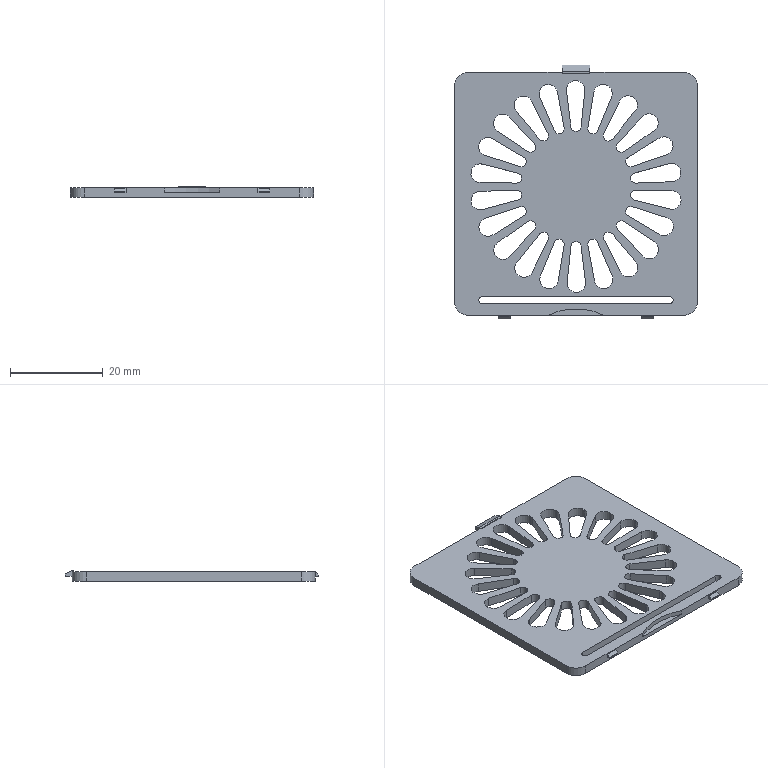Part | SolidWorks | features ICE 4, Extrusion 1, MirrorPattern 1 | 1 solid | 148 faces | box 52.5 x 54.75 x 2.2 mm | volume 3927 mm3 | cylinder 76 | plane 72 | commonest cylinder face diameters 4 x36 2.2 x32 6 x4 1.5 x3 27 x1